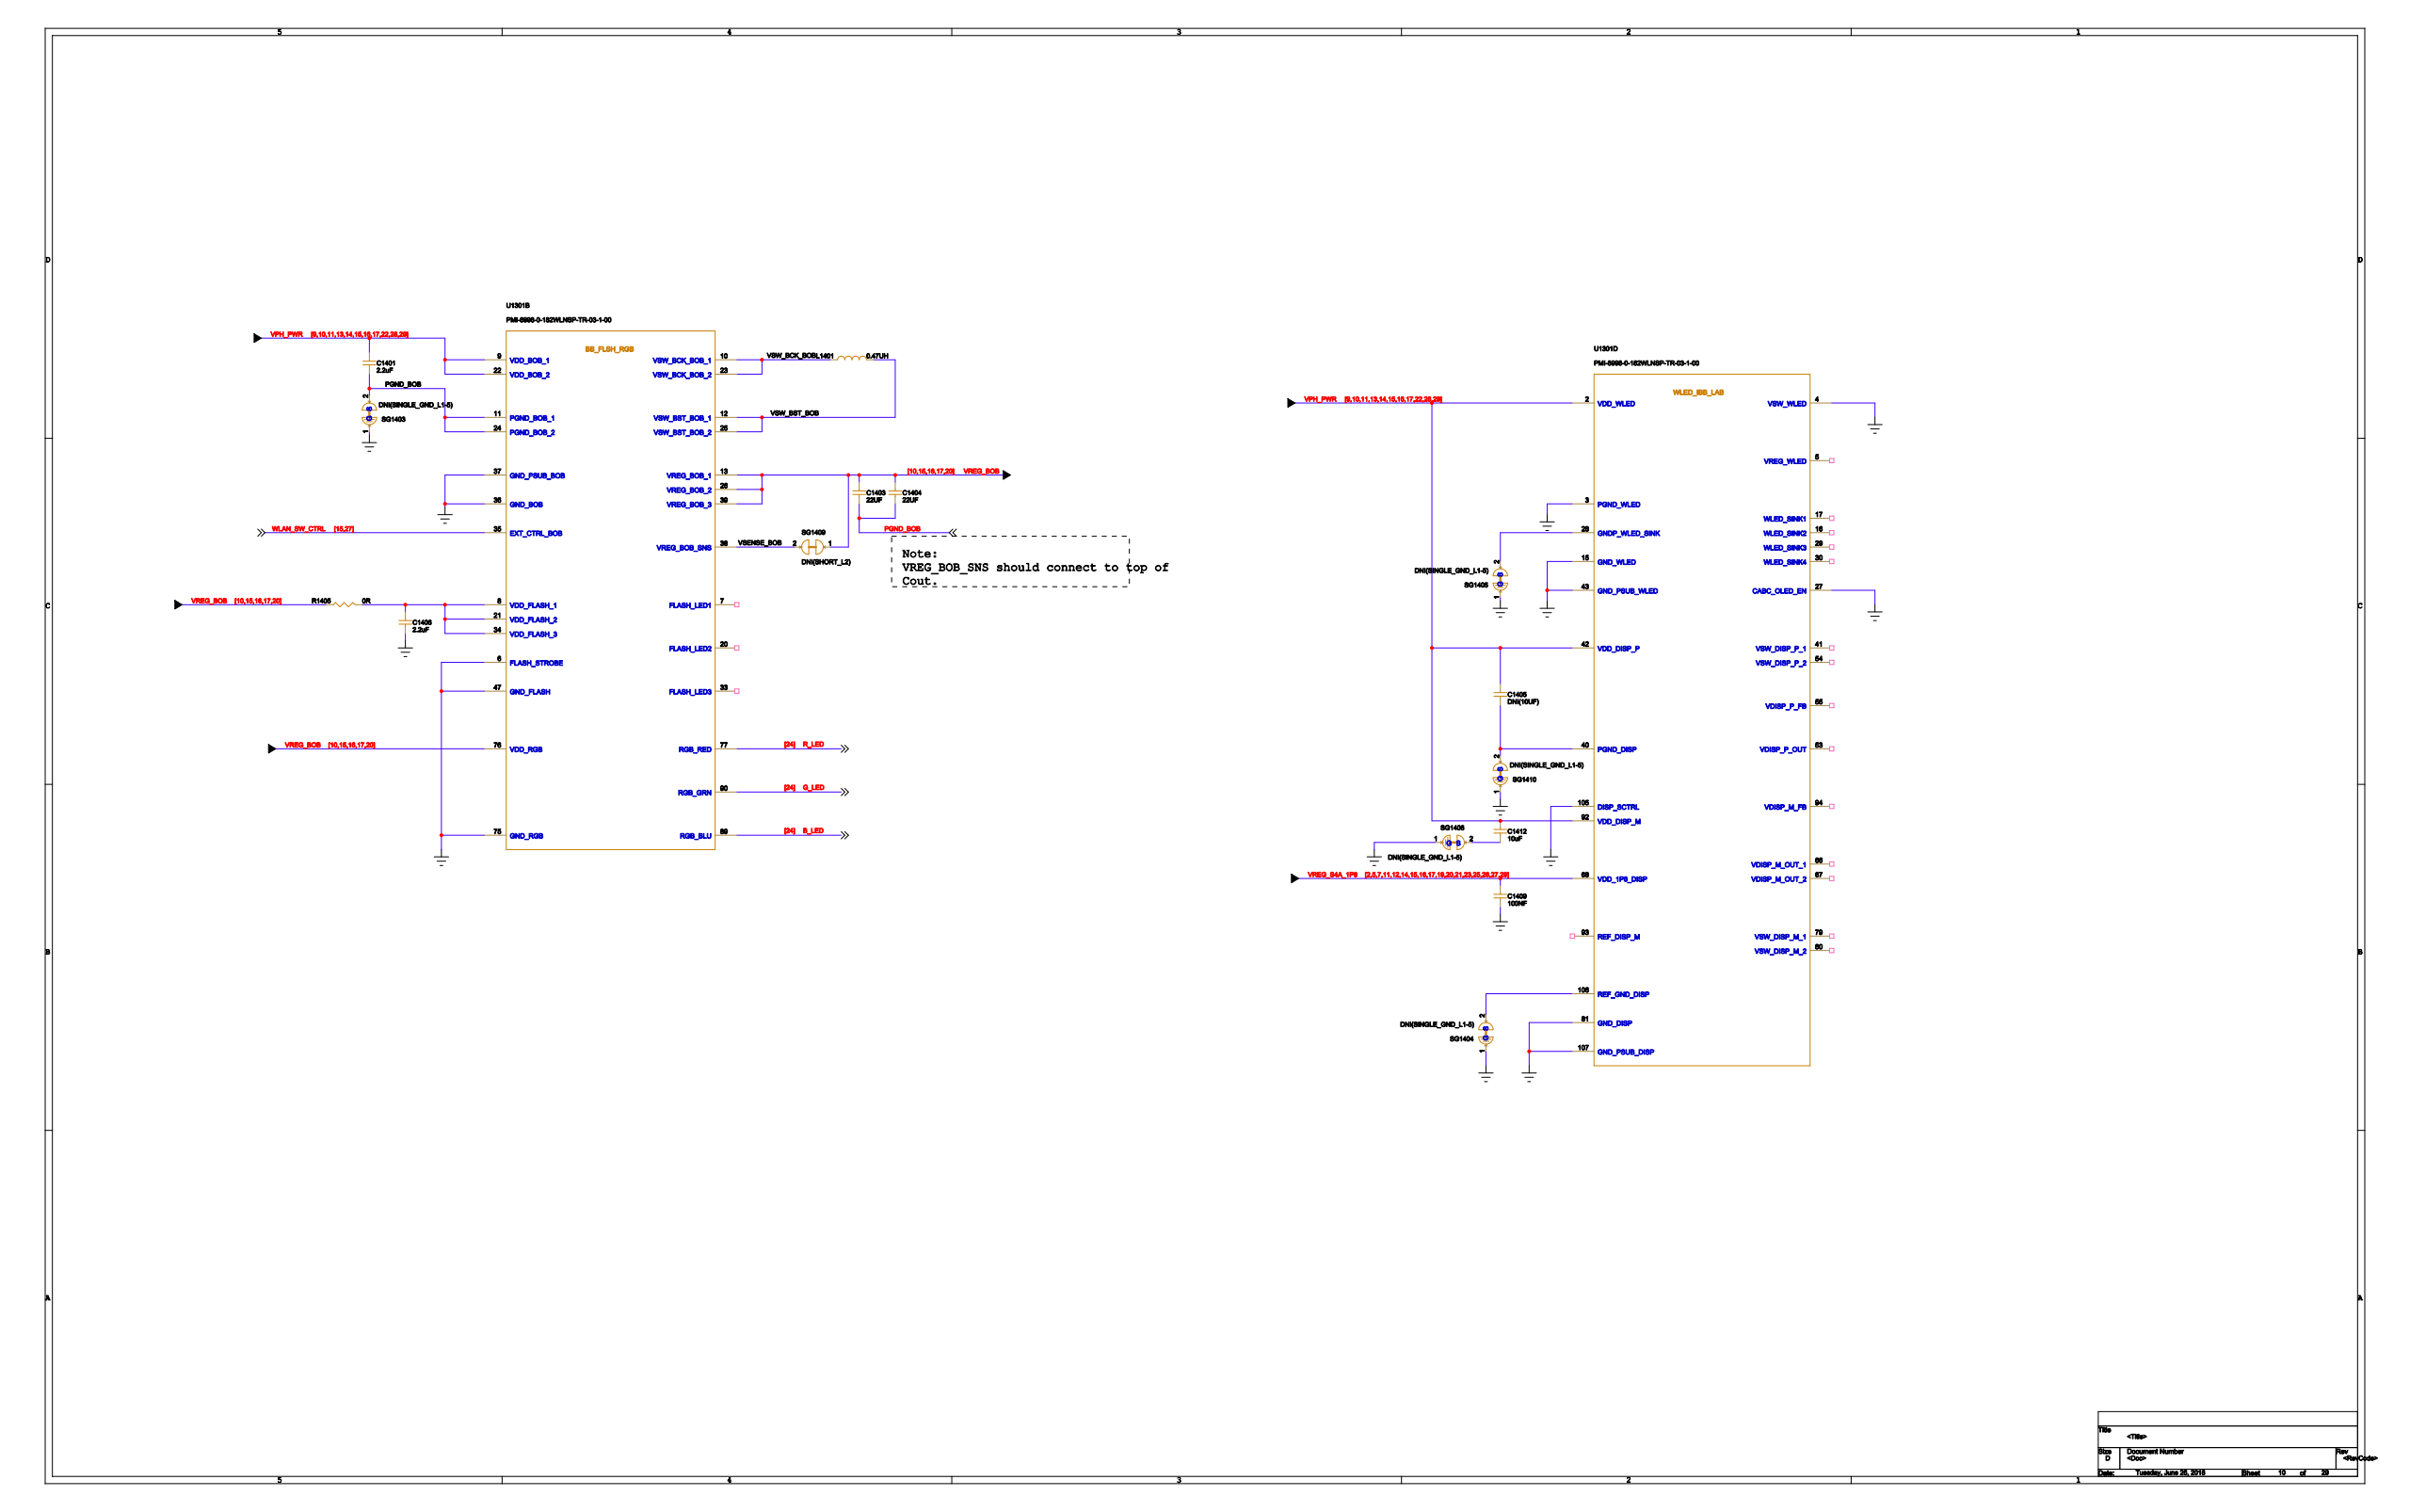Circuit board | Cadence Allegro | 802 parts | 566 nets | one sheet of the schematic
Parts on this sheet (reference | value | footprint):
C1401 | 2.2uF | 0402-BIG
C1403 | 22UF | 0603-BIG
C1404 | 22UF | 0603-BIG
C1405 | DNI(10UF) | 0402-BIG
C1406 | 2.2uF | 0402-BIG
C1409 | 100NF | C0201
C1412 | 10uF | 0402-BIG
L1401 | 0.47UH | L2016_MEKK2016
R1405 | 0R | R0201
SG1403 | DNI(SINGLE_GND_L1-5) | GND_L1-5
SG1404 | DNI(SINGLE_GND_L1-5) | GND_L1-5
SG1405 | DNI(SINGLE_GND_L1-5) | GND_L1-5
SG1408 | DNI(SINGLE_GND_L1-5) | GND_L1-5
SG1409 | DNI(SHORT_L2) | SHORT_L2_2REC08X12
SG1410 | DNI(SINGLE_GND_L1-5) | GND_L1-5
U1301 | PMI-8998-0-182WLNSP-TR-03-1-00 | PMI8998
Nets of these parts (net: part-pin ...):
GND: C1406-2 C1409-2 SG1403-1 SG1404-1 SG1405-1 SG1408-1 SG1410-1 U1301-3 U1301-4 U1301-6 U1301-15 U1301-27 U1301-36 U1301-37 U1301-43 U1301-47 U1301-75 U1301-81 U1301-105 U1301-107
VPH_PWR: C1401-1 C1405-1 C1412-1 U1301-2 U1301-9 U1301-22 U1301-42 U1301-92
N163829: C1412-2 SG1408-2
VREG_S4A_1P8: C1409-1 U1301-68
VREG_BOB: C1403-1 C1404-1 R1405-1 SG1409-1 U1301-13 U1301-26 U1301-39 U1301-76
N159990: C1406-1 R1405-2 U1301-8 U1301-21 U1301-34
PGND_BOB: C1401-2 C1403-2 C1404-2 SG1403-2 U1301-11 U1301-24
N163359: C1405-2 SG1410-2 U1301-40
B_LED: U1301-89
G_LED: U1301-90
R_LED: U1301-77
VSW_BCK_BOB: L1401-1 U1301-10 U1301-23
VSW_BST_BOB: L1401-2 U1301-12 U1301-25
N163631: SG1404-2 U1301-106
N163785: SG1405-2 U1301-28
VSENSE_BOB: SG1409-2 U1301-38
WLAN_SW_CTRL: U1301-35